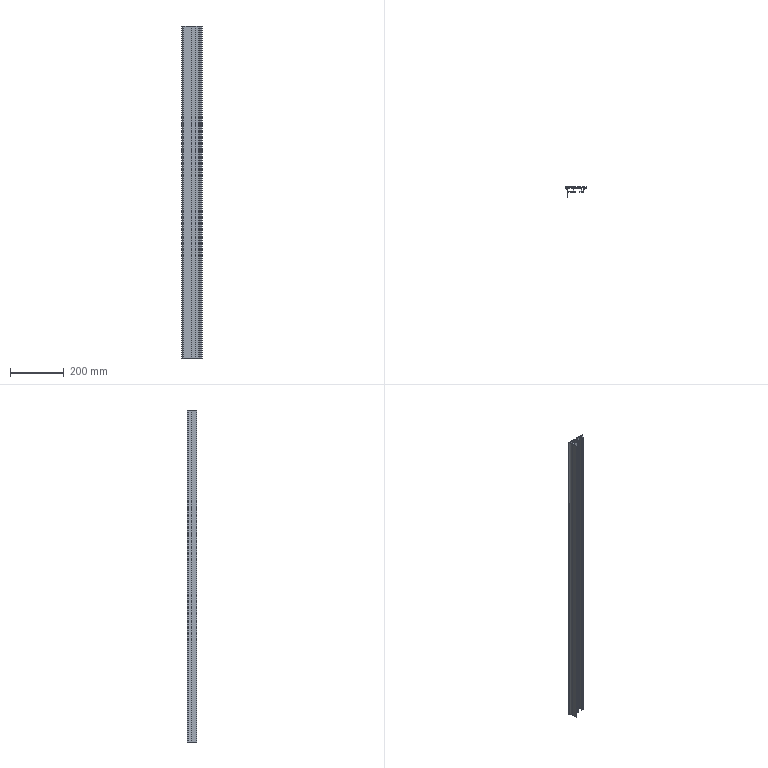Part | STEP file | SIDE | 1 solid | 100 faces | box 76 x 36.5 x 1230 mm | volume 490001 mm3 | plane 72 | cylinder 28 | commonest cylinder face diameters 1 x17 3.625 x4 6 x3 2 x2 40 x1 44 x1